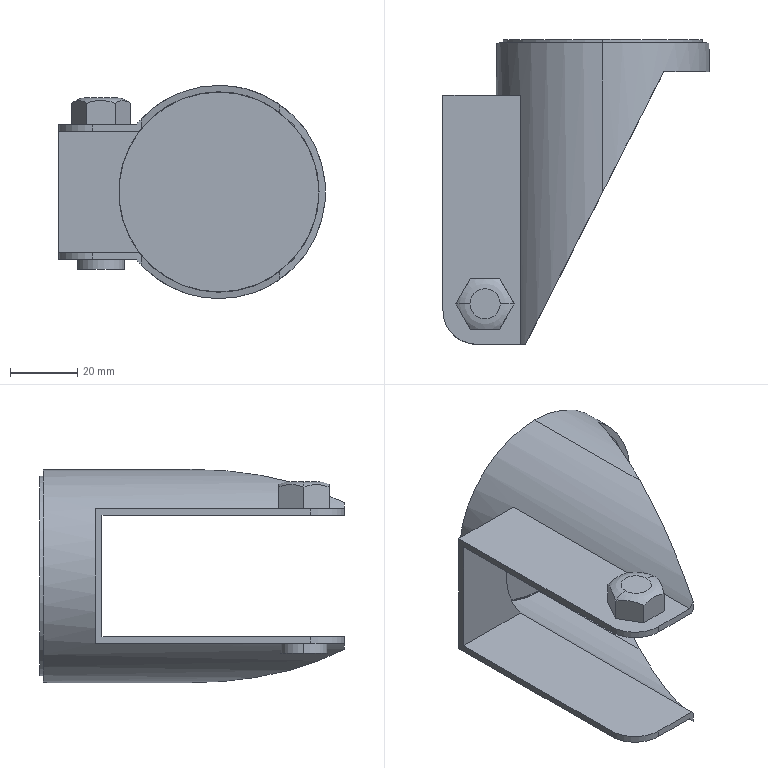Part | SolidWorks | features RefAxis 15, ICE 6, 3DProfileFeature 5, Revolution 2 | 1 solid | 38 faces | box 79.167 x 90.525 x 63.333 mm | volume 28539 mm3 | plane 24 | cylinder 12 | torus 2 | commonest cylinder face diameters 59.333 x4 14 x2 20 x2 59.533 x2 63.333 x2
STEP:
#1=CARTESIAN_POINT('',(-39.5,-94.,28.));
#2=VERTEX_POINT('',#1);
#3=CARTESIAN_POINT('',(-30.5,-94.,28.));
#4=VERTEX_POINT('',#3);
#5=CARTESIAN_POINT('',(-35.,-94.,28.));
#6=DIRECTION('',(0.,0.,-1.));
#7=DIRECTION('',(-1.,0.,0.));
#8=AXIS2_PLACEMENT_3D('',#5,#6,#7);
#9=CIRCLE('',#8,4.5);
#10=EDGE_CURVE('',#2,#4,#9,.T.);
#11=ORIENTED_EDGE('',*,*,#10,.T.);
#12=CARTESIAN_POINT('',(-26.34,-94.,26.33));
#13=VERTEX_POINT('',#12);
#14=CARTESIAN_POINT('',(-30.693,-94.,21.503));
#15=DIRECTION('',(0.,1.,0.));
#16=DIRECTION('',(-1.,0.,0.));
#17=AXIS2_PLACEMENT_3D('',#14,#15,#16);
#18=CIRCLE('',#17,6.5);
#19=EDGE_CURVE('',#4,#13,#18,.T.);
#20=ORIENTED_EDGE('',*,*,#19,.T.);
#21=CARTESIAN_POINT('',(-30.67,-86.5,26.33));
#22=VERTEX_POINT('',#21);
#23=CARTESIAN_POINT('',(-30.67,-86.5,26.33));
#24=CARTESIAN_POINT('',(-30.329,-87.091,26.637));
#25=CARTESIAN_POINT('',(-29.974,-87.705,26.84));
#26=CARTESIAN_POINT('',(-29.429,-88.65,27.038));
#27=CARTESIAN_POINT('',(-29.244,-88.97,27.086));
#28=CARTESIAN_POINT('',(-28.874,-89.611,27.149));
#29=CARTESIAN_POINT('',(-28.689,-89.931,27.164));
#30=CARTESIAN_POINT('',(-28.137,-90.888,27.164));
#31=CARTESIAN_POINT('',(-27.77,-91.522,27.106));
#32=CARTESIAN_POINT('',(-27.225,-92.467,26.909));
#33=CARTESIAN_POINT('',(-27.043,-92.783,26.825));
#34=CARTESIAN_POINT('',(-26.685,-93.402,26.611));
#35=CARTESIAN_POINT('',(-26.51,-93.705,26.483));
#36=CARTESIAN_POINT('',(-26.34,-94.,26.33));
#37=B_SPLINE_CURVE_WITH_KNOTS('',3,(#23,#24,#25,#26,#27,#28,#29,#30,#31,#32,#33,#34,#35,#36),.UNSPECIFIED.,.F.,.F.,(4,2,2,2,2,2,4),(0.00000025,0.002212,0.003318,0.004423,0.006635,0.007741,0.008847),.UNSPECIFIED.);
#38=EDGE_CURVE('',#22,#13,#37,.T.);
#39=ORIENTED_EDGE('',*,*,#38,.F.);
#40=CARTESIAN_POINT('',(-39.33,-86.5,26.33));
#41=VERTEX_POINT('',#40);
#42=CARTESIAN_POINT('',(-39.33,-86.5,26.33));
#43=CARTESIAN_POINT('',(-38.993,-86.5,26.482));
#44=CARTESIAN_POINT('',(-38.645,-86.5,26.61));
#45=CARTESIAN_POINT('',(-37.93,-86.5,26.823));
#46=CARTESIAN_POINT('',(-37.565,-86.5,26.908));
#47=CARTESIAN_POINT('',(-36.833,-86.5,27.04));
#48=CARTESIAN_POINT('',(-36.466,-86.5,27.088));
#49=CARTESIAN_POINT('',(-35.726,-86.5,27.15));
#50=CARTESIAN_POINT('',(-35.351,-86.5,27.165));
#51=CARTESIAN_POINT('',(-34.237,-86.5,27.163));
#52=CARTESIAN_POINT('',(-33.505,-86.5,27.103));
#53=CARTESIAN_POINT('',(-32.424,-86.5,26.906));
#54=CARTESIAN_POINT('',(-32.067,-86.5,26.822));
#55=CARTESIAN_POINT('',(-31.361,-86.5,26.611));
#56=CARTESIAN_POINT('',(-31.009,-86.5,26.483));
#57=CARTESIAN_POINT('',(-30.67,-86.5,26.33));
#58=B_SPLINE_CURVE_WITH_KNOTS('',3,(#42,#43,#44,#45,#46,#47,#48,#49,#50,#51,#52,#53,#54,#55,#56,#57),.UNSPECIFIED.,.F.,.F.,(4,2,2,2,2,2,2,4),(0.0379,0.039,0.0401,0.0412,0.04229,0.04449,0.04559,0.04669),.UNSPECIFIED.);
#59=EDGE_CURVE('',#41,#22,#58,.T.);
#60=ORIENTED_EDGE('',*,*,#59,.F.);
#61=CARTESIAN_POINT('',(-43.66,-94.,26.33));
#62=VERTEX_POINT('',#61);
#63=CARTESIAN_POINT('',(-43.66,-94.,26.33));
#64=CARTESIAN_POINT('',(-43.319,-93.409,26.637));
#65=CARTESIAN_POINT('',(-42.964,-92.795,26.84));
#66=CARTESIAN_POINT('',(-42.419,-91.85,27.038));
#67=CARTESIAN_POINT('',(-42.234,-91.53,27.086));
#68=CARTESIAN_POINT('',(-41.864,-90.889,27.149));
#69=CARTESIAN_POINT('',(-41.679,-90.569,27.164));
#70=CARTESIAN_POINT('',(-41.127,-89.612,27.164));
#71=CARTESIAN_POINT('',(-40.761,-88.978,27.106));
#72=CARTESIAN_POINT('',(-40.215,-88.033,26.909));
#73=CARTESIAN_POINT('',(-40.033,-87.717,26.825));
#74=CARTESIAN_POINT('',(-39.676,-87.098,26.611));
#75=CARTESIAN_POINT('',(-39.501,-86.795,26.483));
#76=CARTESIAN_POINT('',(-39.33,-86.5,26.33));
#77=B_SPLINE_CURVE_WITH_KNOTS('',3,(#63,#64,#65,#66,#67,#68,#69,#70,#71,#72,#73,#74,#75,#76),.UNSPECIFIED.,.F.,.F.,(4,2,2,2,2,2,4),(0.00000025,0.002212,0.003318,0.004423,0.006635,0.007741,0.008847),.UNSPECIFIED.);
#78=EDGE_CURVE('',#62,#41,#77,.T.);
#79=ORIENTED_EDGE('',*,*,#78,.F.);
#80=CARTESIAN_POINT('',(-39.307,-94.,21.503));
#81=DIRECTION('',(0.,-1.,0.));
#82=DIRECTION('',(0.,0.,-1.));
#83=AXIS2_PLACEMENT_3D('',#80,#81,#82);
#84=CIRCLE('',#83,6.5);
#85=EDGE_CURVE('',#2,#62,#84,.T.);
#86=ORIENTED_EDGE('',*,*,#85,.F.);
#87=EDGE_LOOP('',(#11,#20,#39,#60,#79,#86));
#88=FACE_OUTER_BOUND('',#87,.T.);
#89=CARTESIAN_POINT('',(-35.,-94.,21.503));
#90=DIRECTION('',(0.,0.,-1.));
#91=DIRECTION('',(-1.,0.,0.));
#92=AXIS2_PLACEMENT_3D('',#89,#90,#91);
#93=TOROIDAL_SURFACE('',#92,4.307,6.5);
#94=ADVANCED_FACE('',(#88),#93,.T.);
#95=CARTESIAN_POINT('',(-28.,-94.,-23.));
#96=VERTEX_POINT('',#95);
#97=CARTESIAN_POINT('',(-42.,-94.,-23.));
#98=VERTEX_POINT('',#97);
#99=CARTESIAN_POINT('',(-35.,-94.,-23.));
#100=DIRECTION('',(0.,0.,1.));
#101=DIRECTION('',(1.,0.,0.));
#102=AXIS2_PLACEMENT_3D('',#99,#100,#101);
#103=CIRCLE('',#102,7.);
#104=EDGE_CURVE('',#96,#98,#103,.T.);
#105=ORIENTED_EDGE('',*,*,#104,.T.);
#106=CARTESIAN_POINT('',(-42.,-94.,-20.));
#107=VERTEX_POINT('',#106);
#108=CARTESIAN_POINT('',(-42.,-94.,-23.));
#109=DIRECTION('',(0.,0.,1.));
#110=VECTOR('',#109,1000.);
#111=LINE('',#108,#110);
#112=EDGE_CURVE('',#98,#107,#111,.T.);
#113=ORIENTED_EDGE('',*,*,#112,.T.);
#114=CARTESIAN_POINT('',(-28.,-94.,-20.));
#115=VERTEX_POINT('',#114);
#116=CARTESIAN_POINT('',(-35.,-94.,-20.));
#117=DIRECTION('',(0.,0.,-1.));
#118=DIRECTION('',(-1.,0.,0.));
#119=AXIS2_PLACEMENT_3D('',#116,#117,#118);
#120=CIRCLE('',#119,7.);
#121=EDGE_CURVE('',#107,#115,#120,.T.);
#122=ORIENTED_EDGE('',*,*,#121,.T.);
#123=CARTESIAN_POINT('',(-28.,-94.,-23.));
#124=DIRECTION('',(0.,0.,1.));
#125=VECTOR('',#124,1000.);
#126=LINE('',#123,#125);
#127=EDGE_CURVE('',#96,#115,#126,.T.);
#128=ORIENTED_EDGE('',*,*,#127,.F.);
#129=EDGE_LOOP('',(#105,#113,#122,#128));
#130=FACE_OUTER_BOUND('',#129,.T.);
#131=CARTESIAN_POINT('',(-35.,-94.,-23.));
#132=DIRECTION('',(0.,0.,1.));
#133=DIRECTION('',(1.,0.,0.));
#134=AXIS2_PLACEMENT_3D('',#131,#132,#133);
#135=CYLINDRICAL_SURFACE('',#134,7.);
#136=ADVANCED_FACE('',(#130),#135,.T.);
#137=CARTESIAN_POINT('',(0.,-18.475,-29.667));
#138=VERTEX_POINT('',#137);
#139=CARTESIAN_POINT('',(0.,-18.475,29.667));
#140=VERTEX_POINT('',#139);
#141=CARTESIAN_POINT('',(0.,-18.475,0.));
#142=DIRECTION('',(0.,1.,0.));
#143=DIRECTION('',(0.,0.,1.));
#144=AXIS2_PLACEMENT_3D('',#141,#142,#143);
#145=CIRCLE('',#144,29.667);
#146=EDGE_CURVE('',#138,#140,#145,.T.);
#147=ORIENTED_EDGE('',*,*,#146,.F.);
#148=CARTESIAN_POINT('',(0.,-17.975,-29.667));
#149=VERTEX_POINT('',#148);
#150=CARTESIAN_POINT('',(0.,-15.475,-29.667));
#151=DIRECTION('',(0.,1.,0.));
#152=VECTOR('',#151,1000.);
#153=LINE('',#150,#152);
#154=EDGE_CURVE('',#138,#149,#153,.T.);
#155=ORIENTED_EDGE('',*,*,#154,.T.);
#156=CARTESIAN_POINT('',(0.,-17.975,29.667));
#157=VERTEX_POINT('',#156);
#158=CARTESIAN_POINT('',(0.,-17.975,0.));
#159=DIRECTION('',(0.,1.,0.));
#160=DIRECTION('',(0.,0.,1.));
#161=AXIS2_PLACEMENT_3D('',#158,#159,#160);
#162=CIRCLE('',#161,29.667);
#163=EDGE_CURVE('',#149,#157,#162,.T.);
#164=ORIENTED_EDGE('',*,*,#163,.T.);
#165=CARTESIAN_POINT('',(0.,-15.475,29.667));
#166=DIRECTION('',(0.,1.,0.));
#167=VECTOR('',#166,1000.);
#168=LINE('',#165,#167);
#169=EDGE_CURVE('',#140,#157,#168,.T.);
#170=ORIENTED_EDGE('',*,*,#169,.F.);
#171=EDGE_LOOP('',(#147,#155,#164,#170));
#172=FACE_OUTER_BOUND('',#171,.T.);
#173=CARTESIAN_POINT('',(0.,-15.475,0.));
#174=DIRECTION('',(0.,1.,0.));
#175=DIRECTION('',(0.,0.,1.));
#176=AXIS2_PLACEMENT_3D('',#173,#174,#175);
#177=CYLINDRICAL_SURFACE('',#176,29.667);
#178=ADVANCED_FACE('',(#172),#177,.F.);
#179=CARTESIAN_POINT('',(-23.03,-106.,-18.859));
#180=VERTEX_POINT('',#179);
#181=CARTESIAN_POINT('',(0.,-60.626,-29.767));
#182=VERTEX_POINT('',#181);
#183=CARTESIAN_POINT('',(-23.03,-106.,-18.859));
#184=CARTESIAN_POINT('',(-17.28,-94.67,-25.881));
#185=CARTESIAN_POINT('',(-9.077,-78.509,-29.767));
#186=CARTESIAN_POINT('',(0.,-60.626,-29.767));
#187=(BOUNDED_CURVE()B_SPLINE_CURVE(3,(#183,#184,#185,#186),.UNSPECIFIED.,.F.,.F.)B_SPLINE_CURVE_WITH_KNOTS((4,4),(3.828,4.712),.UNSPECIFIED.)CURVE()GEOMETRIC_REPRESENTATION_ITEM()RATIONAL_B_SPLINE_CURVE((1.,0.9358,0.9358,1.))REPRESENTATION_ITEM(''));
#188=EDGE_CURVE('',#180,#182,#187,.T.);
#189=ORIENTED_EDGE('',*,*,#188,.T.);
#190=CARTESIAN_POINT('',(0.,-18.475,-29.767));
#191=VERTEX_POINT('',#190);
#192=CARTESIAN_POINT('',(0.,-162.475,-29.767));
#193=DIRECTION('',(0.,1.,0.));
#194=VECTOR('',#193,1000.);
#195=LINE('',#192,#194);
#196=EDGE_CURVE('',#182,#191,#195,.T.);
#197=ORIENTED_EDGE('',*,*,#196,.T.);
#198=CARTESIAN_POINT('',(0.,-18.475,29.767));
#199=VERTEX_POINT('',#198);
#200=CARTESIAN_POINT('',(0.,-18.475,0.));
#201=DIRECTION('',(0.,1.,0.));
#202=DIRECTION('',(0.,0.,1.));
#203=AXIS2_PLACEMENT_3D('',#200,#201,#202);
#204=CIRCLE('',#203,29.767);
#205=EDGE_CURVE('',#191,#199,#204,.T.);
#206=ORIENTED_EDGE('',*,*,#205,.T.);
#207=CARTESIAN_POINT('',(0.,-60.626,29.767));
#208=VERTEX_POINT('',#207);
#209=CARTESIAN_POINT('',(0.,-162.475,29.767));
#210=DIRECTION('',(0.,1.,0.));
#211=VECTOR('',#210,1000.);
#212=LINE('',#209,#211);
#213=EDGE_CURVE('',#208,#199,#212,.T.);
#214=ORIENTED_EDGE('',*,*,#213,.F.);
#215=CARTESIAN_POINT('',(-23.03,-106.,18.859));
#216=VERTEX_POINT('',#215);
#217=CARTESIAN_POINT('',(0.,-60.626,29.767));
#218=CARTESIAN_POINT('',(-9.077,-78.509,29.767));
#219=CARTESIAN_POINT('',(-17.28,-94.67,25.881));
#220=CARTESIAN_POINT('',(-23.03,-106.,18.859));
#221=(BOUNDED_CURVE()B_SPLINE_CURVE(3,(#217,#218,#219,#220),.UNSPECIFIED.,.F.,.F.)B_SPLINE_CURVE_WITH_KNOTS((4,4),(1.571,2.455),.UNSPECIFIED.)CURVE()GEOMETRIC_REPRESENTATION_ITEM()RATIONAL_B_SPLINE_CURVE((1.,0.9358,0.9358,1.))REPRESENTATION_ITEM(''));
#222=EDGE_CURVE('',#208,#216,#221,.T.);
#223=ORIENTED_EDGE('',*,*,#222,.T.);
#224=CARTESIAN_POINT('',(-23.708,-106.,18.));
#225=VERTEX_POINT('',#224);
#226=CARTESIAN_POINT('',(0.,-106.,0.));
#227=DIRECTION('',(0.,-1.,0.));
#228=DIRECTION('',(0.,0.,1.));
#229=AXIS2_PLACEMENT_3D('',#226,#227,#228);
#230=CIRCLE('',#229,29.767);
#231=EDGE_CURVE('',#216,#225,#230,.T.);
#232=ORIENTED_EDGE('',*,*,#231,.T.);
#233=CARTESIAN_POINT('',(-23.708,-34.,18.));
#234=VERTEX_POINT('',#233);
#235=CARTESIAN_POINT('',(-23.708,-162.475,18.));
#236=DIRECTION('',(0.,-1.,0.));
#237=VECTOR('',#236,1000.);
#238=LINE('',#235,#237);
#239=EDGE_CURVE('',#234,#225,#238,.T.);
#240=ORIENTED_EDGE('',*,*,#239,.F.);
#241=CARTESIAN_POINT('',(-23.708,-34.,-18.));
#242=VERTEX_POINT('',#241);
#243=CARTESIAN_POINT('',(0.,-34.,0.));
#244=DIRECTION('',(0.,1.,0.));
#245=DIRECTION('',(0.,0.,1.));
#246=AXIS2_PLACEMENT_3D('',#243,#244,#245);
#247=CIRCLE('',#246,29.767);
#248=EDGE_CURVE('',#242,#234,#247,.T.);
#249=ORIENTED_EDGE('',*,*,#248,.F.);
#250=CARTESIAN_POINT('',(-23.708,-106.,-18.));
#251=VERTEX_POINT('',#250);
#252=CARTESIAN_POINT('',(-23.708,-162.475,-18.));
#253=DIRECTION('',(0.,1.,0.));
#254=VECTOR('',#253,1000.);
#255=LINE('',#252,#254);
#256=EDGE_CURVE('',#251,#242,#255,.T.);
#257=ORIENTED_EDGE('',*,*,#256,.F.);
#258=CARTESIAN_POINT('',(0.,-106.,0.));
#259=DIRECTION('',(0.,-1.,0.));
#260=DIRECTION('',(0.,0.,1.));
#261=AXIS2_PLACEMENT_3D('',#258,#259,#260);
#262=CIRCLE('',#261,29.767);
#263=EDGE_CURVE('',#251,#180,#262,.T.);
#264=ORIENTED_EDGE('',*,*,#263,.T.);
#265=EDGE_LOOP('',(#189,#197,#206,#214,#223,#232,#240,#249,#257,#264));
#266=FACE_OUTER_BOUND('',#265,.T.);
#267=CARTESIAN_POINT('',(0.,-162.475,0.));
#268=DIRECTION('',(0.,1.,0.));
#269=DIRECTION('',(0.,0.,1.));
#270=AXIS2_PLACEMENT_3D('',#267,#268,#269);
#271=CYLINDRICAL_SURFACE('',#270,29.767);
#272=ADVANCED_FACE('',(#266),#271,.F.);
#273=CARTESIAN_POINT('',(0.,-16.475,29.667));
#274=VERTEX_POINT('',#273);
#275=CARTESIAN_POINT('',(0.,-16.475,-29.667));
#276=VERTEX_POINT('',#275);
#277=CARTESIAN_POINT('',(0.,-16.475,0.));
#278=DIRECTION('',(0.,1.,0.));
#279=DIRECTION('',(0.,0.,1.));
#280=AXIS2_PLACEMENT_3D('',#277,#278,#279);
#281=CIRCLE('',#280,29.667);
#282=EDGE_CURVE('',#274,#276,#281,.T.);
#283=ORIENTED_EDGE('',*,*,#282,.T.);
#284=CARTESIAN_POINT('',(0.,-15.475,-29.667));
#285=VERTEX_POINT('',#284);
#286=CARTESIAN_POINT('',(0.,-15.475,-29.667));
#287=DIRECTION('',(0.,1.,0.));
#288=VECTOR('',#287,1000.);
#289=LINE('',#286,#288);
#290=EDGE_CURVE('',#276,#285,#289,.T.);
#291=ORIENTED_EDGE('',*,*,#290,.T.);
#292=CARTESIAN_POINT('',(0.,-15.475,29.667));
#293=VERTEX_POINT('',#292);
#294=CARTESIAN_POINT('',(0.,-15.475,0.));
#295=DIRECTION('',(0.,1.,0.));
#296=DIRECTION('',(0.,0.,1.));
#297=AXIS2_PLACEMENT_3D('',#294,#295,#296);
#298=CIRCLE('',#297,29.667);
#299=EDGE_CURVE('',#293,#285,#298,.T.);
#300=ORIENTED_EDGE('',*,*,#299,.F.);
#301=CARTESIAN_POINT('',(0.,-15.475,29.667));
#302=DIRECTION('',(0.,1.,0.));
#303=VECTOR('',#302,1000.);
#304=LINE('',#301,#303);
#305=EDGE_CURVE('',#274,#293,#304,.T.);
#306=ORIENTED_EDGE('',*,*,#305,.F.);
#307=EDGE_LOOP('',(#283,#291,#300,#306));
#308=FACE_OUTER_BOUND('',#307,.T.);
#309=CARTESIAN_POINT('',(0.,-15.475,0.));
#310=DIRECTION('',(0.,1.,0.));
#311=DIRECTION('',(0.,0.,1.));
#312=AXIS2_PLACEMENT_3D('',#309,#310,#311);
#313=CYLINDRICAL_SURFACE('',#312,29.667);
#314=ADVANCED_FACE('',(#308),#313,.T.);
#315=CARTESIAN_POINT('',(0.,-60.626,-31.667));
#316=VERTEX_POINT('',#315);
#317=CARTESIAN_POINT('',(18.095,-24.975,-25.987));
#318=VERTEX_POINT('',#317);
#319=CARTESIAN_POINT('',(0.,-60.626,-31.667));
#320=CARTESIAN_POINT('',(6.521,-47.778,-31.667));
#321=CARTESIAN_POINT('',(12.743,-35.519,-29.714));
#322=CARTESIAN_POINT('',(18.095,-24.975,-25.987));
#323=(BOUNDED_CURVE()B_SPLINE_CURVE(3,(#319,#320,#321,#322),.UNSPECIFIED.,.F.,.T.)B_SPLINE_CURVE_WITH_KNOTS((4,4),(4.712,5.321),.UNSPECIFIED.)CURVE()GEOMETRIC_REPRESENTATION_ITEM()RATIONAL_B_SPLINE_CURVE((1.,0.9694,0.9694,1.))REPRESENTATION_ITEM(''));
#324=EDGE_CURVE('',#316,#318,#323,.T.);
#325=ORIENTED_EDGE('',*,*,#324,.F.);
#326=CARTESIAN_POINT('',(0.,-16.475,-31.667));
#327=VERTEX_POINT('',#326);
#328=CARTESIAN_POINT('',(0.,-15.475,-31.667));
#329=DIRECTION('',(0.,1.,0.));
#330=VECTOR('',#329,1000.);
#331=LINE('',#328,#330);
#332=EDGE_CURVE('',#316,#327,#331,.T.);
#333=ORIENTED_EDGE('',*,*,#332,.T.);
#334=CARTESIAN_POINT('',(0.,-16.475,31.667));
#335=VERTEX_POINT('',#334);
#336=CARTESIAN_POINT('',(0.,-16.475,0.));
#337=DIRECTION('',(0.,1.,0.));
#338=DIRECTION('',(0.,0.,1.));
#339=AXIS2_PLACEMENT_3D('',#336,#337,#338);
#340=CIRCLE('',#339,31.667);
#341=EDGE_CURVE('',#335,#327,#340,.T.);
#342=ORIENTED_EDGE('',*,*,#341,.F.);
#343=CARTESIAN_POINT('',(0.,-60.626,31.667));
#344=VERTEX_POINT('',#343);
#345=CARTESIAN_POINT('',(0.,-15.475,31.667));
#346=DIRECTION('',(0.,1.,0.));
#347=VECTOR('',#346,1000.);
#348=LINE('',#345,#347);
#349=EDGE_CURVE('',#344,#335,#348,.T.);
#350=ORIENTED_EDGE('',*,*,#349,.F.);
#351=CARTESIAN_POINT('',(18.095,-24.975,25.987));
#352=VERTEX_POINT('',#351);
#353=CARTESIAN_POINT('',(18.095,-24.975,25.987));
#354=CARTESIAN_POINT('',(12.743,-35.519,29.714));
#355=CARTESIAN_POINT('',(6.521,-47.778,31.667));
#356=CARTESIAN_POINT('',(0.,-60.626,31.667));
#357=(BOUNDED_CURVE()B_SPLINE_CURVE(3,(#353,#354,#355,#356),.UNSPECIFIED.,.F.,.F.)B_SPLINE_CURVE_WITH_KNOTS((4,4),(0.9626,1.571),.UNSPECIFIED.)CURVE()GEOMETRIC_REPRESENTATION_ITEM()RATIONAL_B_SPLINE_CURVE((1.,0.9694,0.9694,1.))REPRESENTATION_ITEM(''));
#358=EDGE_CURVE('',#352,#344,#357,.T.);
#359=ORIENTED_EDGE('',*,*,#358,.F.);
#360=CARTESIAN_POINT('',(0.,-24.975,0.));
#361=DIRECTION('',(0.,-1.,0.));
#362=DIRECTION('',(-1.,0.,0.));
#363=AXIS2_PLACEMENT_3D('',#360,#361,#362);
#364=CIRCLE('',#363,31.667);
#365=EDGE_CURVE('',#318,#352,#364,.T.);
#366=ORIENTED_EDGE('',*,*,#365,.F.);
#367=EDGE_LOOP('',(#325,#333,#342,#350,#359,#366));
#368=FACE_OUTER_BOUND('',#367,.T.);
#369=CARTESIAN_POINT('',(0.,-15.475,0.));
#370=DIRECTION('',(0.,1.,0.));
#371=DIRECTION('',(0.,0.,1.));
#372=AXIS2_PLACEMENT_3D('',#369,#370,#371);
#373=CYLINDRICAL_SURFACE('',#372,31.667);
#374=ADVANCED_FACE('',(#368),#373,.T.);
#375=CARTESIAN_POINT('',(-47.5,-32.,-20.));
#376=VERTEX_POINT('',#375);
#377=CARTESIAN_POINT('',(-47.5,-32.,20.));
#378=VERTEX_POINT('',#377);
#379=CARTESIAN_POINT('',(-47.5,-32.,-20.));
#380=DIRECTION('',(0.,0.,1.));
#381=VECTOR('',#380,1000.);
#382=LINE('',#379,#381);
#383=EDGE_CURVE('',#376,#378,#382,.T.);
#384=ORIENTED_EDGE('',*,*,#383,.F.);
#385=CARTESIAN_POINT('',(-47.5,-96.,-20.));
#386=VERTEX_POINT('',#385);
#387=CARTESIAN_POINT('',(-47.5,-106.,-20.));
#388=DIRECTION('',(0.,1.,0.));
#389=VECTOR('',#388,1000.);
#390=LINE('',#387,#389);
#391=EDGE_CURVE('',#386,#376,#390,.T.);
#392=ORIENTED_EDGE('',*,*,#391,.F.);
#393=CARTESIAN_POINT('',(-47.5,-96.,-18.));
#394=VERTEX_POINT('',#393);
#395=CARTESIAN_POINT('',(-47.5,-96.,-95.));
#396=DIRECTION('',(0.,0.,1.));
#397=VECTOR('',#396,1000.);
#398=LINE('',#395,#397);
#399=EDGE_CURVE('',#386,#394,#398,.T.);
#400=ORIENTED_EDGE('',*,*,#399,.T.);
#401=CARTESIAN_POINT('',(-47.5,-34.,-18.));
#402=VERTEX_POINT('',#401);
#403=CARTESIAN_POINT('',(-47.5,-34.,-18.));
#404=DIRECTION('',(0.,-1.,0.));
#405=VECTOR('',#404,1000.);
#406=LINE('',#403,#405);
#407=EDGE_CURVE('',#402,#394,#406,.T.);
#408=ORIENTED_EDGE('',*,*,#407,.F.);
#409=CARTESIAN_POINT('',(-47.5,-34.,18.));
#410=VERTEX_POINT('',#409);
#411=CARTESIAN_POINT('',(-47.5,-34.,18.));
#412=DIRECTION('',(0.,0.,-1.));
#413=VECTOR('',#412,1000.);
#414=LINE('',#411,#413);
#415=EDGE_CURVE('',#410,#402,#414,.T.);
#416=ORIENTED_EDGE('',*,*,#415,.F.);
#417=CARTESIAN_POINT('',(-47.5,-96.,18.));
#418=VERTEX_POINT('',#417);
#419=CARTESIAN_POINT('',(-47.5,-106.,18.));
#420=DIRECTION('',(0.,1.,0.));
#421=VECTOR('',#420,1000.);
#422=LINE('',#419,#421);
#423=EDGE_CURVE('',#418,#410,#422,.T.);
#424=ORIENTED_EDGE('',*,*,#423,.F.);
#425=CARTESIAN_POINT('',(-47.5,-96.,20.));
#426=VERTEX_POINT('',#425);
#427=CARTESIAN_POINT('',(-47.5,-96.,-95.));
#428=DIRECTION('',(0.,0.,1.));
#429=VECTOR('',#428,1000.);
#430=LINE('',#427,#429);
#431=EDGE_CURVE('',#418,#426,#430,.T.);
#432=ORIENTED_EDGE('',*,*,#431,.T.);
#433=CARTESIAN_POINT('',(-47.5,-32.,20.));
#434=DIRECTION('',(0.,-1.,0.));
#435=VECTOR('',#434,1000.);
#436=LINE('',#433,#435);
#437=EDGE_CURVE('',#378,#426,#436,.T.);
#438=ORIENTED_EDGE('',*,*,#437,.F.);
#439=EDGE_LOOP('',(#384,#392,#400,#408,#416,#424,#432,#438));
#440=FACE_OUTER_BOUND('',#439,.T.);
#441=CARTESIAN_POINT('',(-47.5,0.,0.));
#442=DIRECTION('',(1.,0.,0.));
#443=DIRECTION('',(0.,0.,-1.));
#444=AXIS2_PLACEMENT_3D('',#441,#442,#443);
#445=PLANE('',#444);
#446=ADVANCED_FACE('',(#440),#445,.F.);
#447=CARTESIAN_POINT('',(-37.5,-106.,20.));
#448=VERTEX_POINT('',#447);
#449=CARTESIAN_POINT('',(-24.552,-106.,20.));
#450=VERTEX_POINT('',#449);
#451=CARTESIAN_POINT('',(-47.5,-106.,20.));
#452=DIRECTION('',(1.,0.,0.));
#453=VECTOR('',#452,1000.);
#454=LINE('',#451,#453);
#455=EDGE_CURVE('',#448,#450,#454,.T.);
#456=ORIENTED_EDGE('',*,*,#455,.F.);
#457=CARTESIAN_POINT('',(-37.5,-106.,18.));
#458=VERTEX_POINT('',#457);
#459=CARTESIAN_POINT('',(-37.5,-106.,-95.));
#460=DIRECTION('',(0.,0.,1.));
#461=VECTOR('',#460,1000.);
#462=LINE('',#459,#461);
#463=EDGE_CURVE('',#458,#448,#462,.T.);
#464=ORIENTED_EDGE('',*,*,#463,.F.);
#465=CARTESIAN_POINT('',(-47.5,-106.,18.));
#466=DIRECTION('',(1.,0.,0.));
#467=VECTOR('',#466,1000.);
#468=LINE('',#465,#467);
#469=EDGE_CURVE('',#458,#225,#468,.T.);
#470=ORIENTED_EDGE('',*,*,#469,.T.);
#471=ORIENTED_EDGE('',*,*,#231,.F.);
#472=CARTESIAN_POINT('',(-23.03,-106.,21.734));
#473=VERTEX_POINT('',#472);
#474=CARTESIAN_POINT('',(-23.03,-106.,-95.));
#475=DIRECTION('',(0.,0.,1.));
#476=VECTOR('',#475,1000.);
#477=LINE('',#474,#476);
#478=EDGE_CURVE('',#216,#473,#477,.T.);
#479=ORIENTED_EDGE('',*,*,#478,.T.);
#480=CARTESIAN_POINT('',(0.,-106.,0.));
#481=DIRECTION('',(0.,-1.,0.));
#482=DIRECTION('',(0.,0.,1.));
#483=AXIS2_PLACEMENT_3D('',#480,#481,#482);
#484=CIRCLE('',#483,31.667);
#485=EDGE_CURVE('',#473,#450,#484,.T.);
#486=ORIENTED_EDGE('',*,*,#485,.T.);
#487=EDGE_LOOP('',(#456,#464,#470,#471,#479,#486));
#488=FACE_OUTER_BOUND('',#487,.T.);
#489=CARTESIAN_POINT('',(-47.5,-106.,20.));
#490=DIRECTION('',(0.,-1.,0.));
#491=DIRECTION('',(0.,0.,-1.));
#492=AXIS2_PLACEMENT_3D('',#489,#490,#491);
#493=PLANE('',#492);
#494=ADVANCED_FACE('',(#488),#493,.T.);
#495=CARTESIAN_POINT('',(-37.5,-106.,-18.));
#496=VERTEX_POINT('',#495);
#497=CARTESIAN_POINT('',(-47.5,-106.,-18.));
#498=DIRECTION('',(1.,0.,0.));
#499=VECTOR('',#498,1000.);
#500=LINE('',#497,#499);
#501=EDGE_CURVE('',#496,#251,#500,.T.);
#502=ORIENTED_EDGE('',*,*,#501,.F.);
#503=CARTESIAN_POINT('',(-37.5,-106.,-20.));
#504=VERTEX_POINT('',#503);
#505=CARTESIAN_POINT('',(-37.5,-106.,-95.));
#506=DIRECTION('',(0.,0.,1.));
#507=VECTOR('',#506,1000.);
#508=LINE('',#505,#507);
#509=EDGE_CURVE('',#504,#496,#508,.T.);
#510=ORIENTED_EDGE('',*,*,#509,.F.);
#511=CARTESIAN_POINT('',(-24.552,-106.,-20.));
#512=VERTEX_POINT('',#511);
#513=CARTESIAN_POINT('',(-47.5,-106.,-20.));
#514=DIRECTION('',(1.,0.,0.));
#515=VECTOR('',#514,1000.);
#516=LINE('',#513,#515);
#517=EDGE_CURVE('',#504,#512,#516,.T.);
#518=ORIENTED_EDGE('',*,*,#517,.T.);
#519=CARTESIAN_POINT('',(-23.03,-106.,-21.734));
#520=VERTEX_POINT('',#519);
#521=CARTESIAN_POINT('',(0.,-106.,0.));
#522=DIRECTION('',(0.,-1.,0.));
#523=DIRECTION('',(0.,0.,1.));
#524=AXIS2_PLACEMENT_3D('',#521,#522,#523);
#525=CIRCLE('',#524,31.667);
#526=EDGE_CURVE('',#512,#520,#525,.T.);
#527=ORIENTED_EDGE('',*,*,#526,.T.);
#528=CARTESIAN_POINT('',(-23.03,-106.,-95.));
#529=DIRECTION('',(0.,0.,1.));
#530=VECTOR('',#529,1000.);
#531=LINE('',#528,#530);
#532=EDGE_CURVE('',#520,#180,#531,.T.);
#533=ORIENTED_EDGE('',*,*,#532,.T.);
#534=ORIENTED_EDGE('',*,*,#263,.F.);
#535=EDGE_LOOP('',(#502,#510,#518,#527,#533,#534));
#536=FACE_OUTER_BOUND('',#535,.T.);
#537=CARTESIAN_POINT('',(-47.5,-106.,-18.));
#538=DIRECTION('',(0.,-1.,0.));
#539=DIRECTION('',(0.,0.,-1.));
#540=AXIS2_PLACEMENT_3D('',#537,#538,#539);
#541=PLANE('',#540);
#542=ADVANCED_FACE('',(#536),#541,.T.);
#543=ORIENTED_EDGE('',*,*,#332,.F.);
#544=CARTESIAN_POINT('',(-23.03,-106.,-21.734));
#545=CARTESIAN_POINT('',(-16.961,-94.043,-28.165));
#546=CARTESIAN_POINT('',(-8.842,-78.047,-31.667));
#547=CARTESIAN_POINT('',(0.,-60.626,-31.667));
#548=(BOUNDED_CURVE()B_SPLINE_CURVE(3,(#544,#545,#546,#547),.UNSPECIFIED.,.F.,.T.)B_SPLINE_CURVE_WITH_KNOTS((4,4),(3.898,4.712),.UNSPECIFIED.)CURVE()GEOMETRIC_REPRESENTATION_ITEM()RATIONAL_B_SPLINE_CURVE((1.,0.9455,0.9455,1.))REPRESENTATION_ITEM(''));
#549=EDGE_CURVE('',#520,#316,#548,.T.);
#550=ORIENTED_EDGE('',*,*,#549,.F.);
#551=ORIENTED_EDGE('',*,*,#526,.F.);
#552=CARTESIAN_POINT('',(-24.552,-32.,-20.));
#553=VERTEX_POINT('',#552);
#554=CARTESIAN_POINT('',(-24.552,-15.475,-20.));
#555=DIRECTION('',(0.,-1.,0.));
#556=VECTOR('',#555,1000.);
#557=LINE('',#554,#556);
#558=EDGE_CURVE('',#553,#512,#557,.T.);
#559=ORIENTED_EDGE('',*,*,#558,.F.);
#560=CARTESIAN_POINT('',(-24.552,-32.,20.));
#561=VERTEX_POINT('',#560);
#562=CARTESIAN_POINT('',(0.,-32.,0.));
#563=DIRECTION('',(0.,-1.,0.));
#564=DIRECTION('',(0.,0.,1.));
#565=AXIS2_PLACEMENT_3D('',#562,#563,#564);
#566=CIRCLE('',#565,31.667);
#567=EDGE_CURVE('',#561,#553,#566,.T.);
#568=ORIENTED_EDGE('',*,*,#567,.F.);
#569=CARTESIAN_POINT('',(-24.552,-15.475,20.));
#570=DIRECTION('',(0.,1.,0.));
#571=VECTOR('',#570,1000.);
#572=LINE('',#569,#571);
#573=EDGE_CURVE('',#450,#561,#572,.T.);
#574=ORIENTED_EDGE('',*,*,#573,.F.);
#575=ORIENTED_EDGE('',*,*,#485,.F.);
#576=CARTESIAN_POINT('',(0.,-60.626,31.667));
#577=CARTESIAN_POINT('',(-8.842,-78.047,31.667));
#578=CARTESIAN_POINT('',(-16.961,-94.043,28.165));
#579=CARTESIAN_POINT('',(-23.03,-106.,21.734));
#580=(BOUNDED_CURVE()B_SPLINE_CURVE(3,(#576,#577,#578,#579),.UNSPECIFIED.,.F.,.F.)B_SPLINE_CURVE_WITH_KNOTS((4,4),(1.571,2.385),.UNSPECIFIED.)CURVE()GEOMETRIC_REPRESENTATION_ITEM()RATIONAL_B_SPLINE_CURVE((1.,0.9455,0.9455,1.))REPRESENTATION_ITEM(''));
#581=EDGE_CURVE('',#344,#473,#580,.T.);
#582=ORIENTED_EDGE('',*,*,#581,.F.);
#583=ORIENTED_EDGE('',*,*,#349,.T.);
#584=CARTESIAN_POINT('',(0.,-16.475,0.));
#585=DIRECTION('',(0.,1.,0.));
#586=DIRECTION('',(0.,0.,1.));
#587=AXIS2_PLACEMENT_3D('',#584,#585,#586);
#588=CIRCLE('',#587,31.667);
#589=EDGE_CURVE('',#327,#335,#588,.T.);
#590=ORIENTED_EDGE('',*,*,#589,.F.);
#591=EDGE_LOOP('',(#543,#550,#551,#559,#568,#574,#575,#582,#583,#590));
#592=FACE_OUTER_BOUND('',#591,.T.);
#593=CARTESIAN_POINT('',(0.,-15.475,0.));
#594=DIRECTION('',(0.,1.,0.));
#595=DIRECTION('',(0.,0.,1.));
#596=AXIS2_PLACEMENT_3D('',#593,#594,#595);
#597=CYLINDRICAL_SURFACE('',#596,31.667);
#598=ADVANCED_FACE('',(#592),#597,.T.);
#599=ORIENTED_EDGE('',*,*,#341,.T.);
#600=ORIENTED_EDGE('',*,*,#589,.T.);
#601=EDGE_LOOP('',(#599,#600));
#602=FACE_OUTER_BOUND('',#601,.T.);
#603=ORIENTED_EDGE('',*,*,#282,.F.);
#604=CARTESIAN_POINT('',(0.,-16.475,0.));
#605=DIRECTION('',(0.,1.,0.));
#606=DIRECTION('',(0.,0.,1.));
#607=AXIS2_PLACEMENT_3D('',#604,#605,#606);
#608=CIRCLE('',#607,29.667);
#609=EDGE_CURVE('',#276,#274,#608,.T.);
#610=ORIENTED_EDGE('',*,*,#609,.F.);
#611=EDGE_LOOP('',(#603,#610));
#612=FACE_BOUND('',#611,.T.);
#613=CARTESIAN_POINT('',(0.,-16.475,31.667));
#614=DIRECTION('',(0.,1.,0.));
#615=DIRECTION('',(0.,0.,1.));
#616=AXIS2_PLACEMENT_3D('',#613,#614,#615);
#617=PLANE('',#616);
#618=ADVANCED_FACE('',(#602,#612),#617,.T.);
#619=ORIENTED_EDGE('',*,*,#290,.F.);
#620=ORIENTED_EDGE('',*,*,#609,.T.);
#621=ORIENTED_EDGE('',*,*,#305,.T.);
#622=CARTESIAN_POINT('',(0.,-15.475,0.));
#623=DIRECTION('',(0.,1.,0.));
#624=DIRECTION('',(0.,0.,1.));
#625=AXIS2_PLACEMENT_3D('',#622,#623,#624);
#626=CIRCLE('',#625,29.667);
#627=EDGE_CURVE('',#285,#293,#626,.T.);
#628=ORIENTED_EDGE('',*,*,#627,.F.);
#629=EDGE_LOOP('',(#619,#620,#621,#628));
#630=FACE_OUTER_BOUND('',#629,.T.);
#631=CARTESIAN_POINT('',(0.,-15.475,0.));
#632=DIRECTION('',(0.,1.,0.));
#633=DIRECTION('',(0.,0.,1.));
#634=AXIS2_PLACEMENT_3D('',#631,#632,#633);
#635=CYLINDRICAL_SURFACE('',#634,29.667);
#636=ADVANCED_FACE('',(#630),#635,.T.);
#637=ORIENTED_EDGE('',*,*,#299,.T.);
#638=ORIENTED_EDGE('',*,*,#627,.T.);
#639=EDGE_LOOP('',(#637,#638));
#640=FACE_OUTER_BOUND('',#639,.T.);
#641=CARTESIAN_POINT('',(0.,-15.475,29.667));
#642=DIRECTION('',(0.,1.,0.));
#643=DIRECTION('',(0.,0.,1.));
#644=AXIS2_PLACEMENT_3D('',#641,#642,#643);
#645=PLANE('',#644);
#646=ADVANCED_FACE('',(#640),#645,.T.);
#647=CARTESIAN_POINT('',(-95.,-34.,-18.));
#648=DIRECTION('',(1.,0.,0.));
#649=VECTOR('',#648,1000.);
#650=LINE('',#647,#649);
#651=EDGE_CURVE('',#402,#242,#650,.T.);
#652=ORIENTED_EDGE('',*,*,#651,.T.);
#653=ORIENTED_EDGE('',*,*,#248,.T.);
#654=CARTESIAN_POINT('',(-95.,-34.,18.));
#655=DIRECTION('',(1.,0.,0.));
#656=VECTOR('',#655,1000.);
#657=LINE('',#654,#656);
#658=EDGE_CURVE('',#410,#234,#657,.T.);
#659=ORIENTED_EDGE('',*,*,#658,.F.);
#660=ORIENTED_EDGE('',*,*,#415,.T.);
#661=EDGE_LOOP('',(#652,#653,#659,#660));
#662=FACE_OUTER_BOUND('',#661,.T.);
#663=CARTESIAN_POINT('',(-95.,-34.,-18.));
#664=DIRECTION('',(0.,1.,0.));
#665=DIRECTION('',(0.,0.,1.));
#666=AXIS2_PLACEMENT_3D('',#663,#664,#665);
#667=PLANE('',#666);
#668=ADVANCED_FACE('',(#662),#667,.F.);
#669=ORIENTED_EDGE('',*,*,#407,.T.);
#670=CARTESIAN_POINT('',(-37.5,-96.,-18.));
#671=DIRECTION('',(0.,0.,1.));
#672=DIRECTION('',(-1.,0.,0.));
#673=AXIS2_PLACEMENT_3D('',#670,#671,#672);
#674=CIRCLE('',#673,10.);
#675=EDGE_CURVE('',#394,#496,#674,.T.);
#676=ORIENTED_EDGE('',*,*,#675,.T.);
#677=ORIENTED_EDGE('',*,*,#501,.T.);
#678=ORIENTED_EDGE('',*,*,#256,.T.);
#679=ORIENTED_EDGE('',*,*,#651,.F.);
#680=EDGE_LOOP('',(#669,#676,#677,#678,#679));
#681=FACE_OUTER_BOUND('',#680,.T.);
#682=CARTESIAN_POINT('',(-95.,-140.,-18.));
#683=DIRECTION('',(0.,0.,-1.));
#684=DIRECTION('',(-1.,0.,0.));
#685=AXIS2_PLACEMENT_3D('',#682,#683,#684);
#686=PLANE('',#685);
#687=ADVANCED_FACE('',(#681),#686,.F.);
#688=ORIENTED_EDGE('',*,*,#469,.F.);
#689=CARTESIAN_POINT('',(-37.5,-96.,18.));
#690=DIRECTION('',(0.,0.,-1.));
#691=DIRECTION('',(1.,0.,0.));
#692=AXIS2_PLACEMENT_3D('',#689,#690,#691);
#693=CIRCLE('',#692,10.);
#694=EDGE_CURVE('',#458,#418,#693,.T.);
#695=ORIENTED_EDGE('',*,*,#694,.T.);
#696=ORIENTED_EDGE('',*,*,#423,.T.);
#697=ORIENTED_EDGE('',*,*,#658,.T.);
#698=ORIENTED_EDGE('',*,*,#239,.T.);
#699=EDGE_LOOP('',(#688,#695,#696,#697,#698));
#700=FACE_OUTER_BOUND('',#699,.T.);
#701=CARTESIAN_POINT('',(-95.,-34.,18.));
#702=DIRECTION('',(0.,0.,1.));
#703=DIRECTION('',(1.,0.,0.));
#704=AXIS2_PLACEMENT_3D('',#701,#702,#703);
#705=PLANE('',#704);
#706=ADVANCED_FACE('',(#700),#705,.F.);
#707=CARTESIAN_POINT('',(-37.5,-96.,20.));
#708=DIRECTION('',(0.,0.,-1.));
#709=DIRECTION('',(1.,0.,0.));
#710=AXIS2_PLACEMENT_3D('',#707,#708,#709);
#711=CIRCLE('',#710,10.);
#712=EDGE_CURVE('',#448,#426,#711,.T.);
#713=ORIENTED_EDGE('',*,*,#712,.F.);
#714=ORIENTED_EDGE('',*,*,#455,.T.);
#715=ORIENTED_EDGE('',*,*,#573,.T.);
#716=CARTESIAN_POINT('',(-47.5,-32.,20.));
#717=DIRECTION('',(1.,0.,0.));
#718=VECTOR('',#717,1000.);
#719=LINE('',#716,#718);
#720=EDGE_CURVE('',#378,#561,#719,.T.);
#721=ORIENTED_EDGE('',*,*,#720,.F.);
#722=ORIENTED_EDGE('',*,*,#437,.T.);
#723=EDGE_LOOP('',(#713,#714,#715,#721,#722));
#724=FACE_OUTER_BOUND('',#723,.T.);
#725=CARTESIAN_POINT('',(-39.33,-86.5,20.));
#726=VERTEX_POINT('',#725);
#727=CARTESIAN_POINT('',(-43.66,-94.,20.));
#728=VERTEX_POINT('',#727);
#729=CARTESIAN_POINT('',(-39.33,-86.5,20.));
#730=DIRECTION('',(-0.5,-0.866,0.));
#731=VECTOR('',#730,1000.);
#732=LINE('',#729,#731);
#733=EDGE_CURVE('',#726,#728,#732,.T.);
#734=ORIENTED_EDGE('',*,*,#733,.F.);
#735=CARTESIAN_POINT('',(-30.67,-86.5,20.));
#736=VERTEX_POINT('',#735);
#737=CARTESIAN_POINT('',(-30.67,-86.5,20.));
#738=DIRECTION('',(-1.,0.,0.));
#739=VECTOR('',#738,1000.);
#740=LINE('',#737,#739);
#741=EDGE_CURVE('',#736,#726,#740,.T.);
#742=ORIENTED_EDGE('',*,*,#741,.F.);
#743=CARTESIAN_POINT('',(-26.34,-94.,20.));
#744=VERTEX_POINT('',#743);
#745=CARTESIAN_POINT('',(-26.34,-94.,20.));
#746=DIRECTION('',(-0.5,0.866,0.));
#747=VECTOR('',#746,1000.);
#748=LINE('',#745,#747);
#749=EDGE_CURVE('',#744,#736,#748,.T.);
#750=ORIENTED_EDGE('',*,*,#749,.F.);
#751=CARTESIAN_POINT('',(-30.67,-101.5,20.));
#752=VERTEX_POINT('',#751);
#753=CARTESIAN_POINT('',(-30.67,-101.5,20.));
#754=DIRECTION('',(0.5,0.866,0.));
#755=VECTOR('',#754,1000.);
#756=LINE('',#753,#755);
#757=EDGE_CURVE('',#752,#744,#756,.T.);
#758=ORIENTED_EDGE('',*,*,#757,.F.);
#759=CARTESIAN_POINT('',(-39.33,-101.5,20.));
#760=VERTEX_POINT('',#759);
#761=CARTESIAN_POINT('',(-39.33,-101.5,20.));
#762=DIRECTION('',(1.,0.,0.));
#763=VECTOR('',#762,1000.);
#764=LINE('',#761,#763);
#765=EDGE_CURVE('',#760,#752,#764,.T.);
#766=ORIENTED_EDGE('',*,*,#765,.F.);
#767=CARTESIAN_POINT('',(-43.66,-94.,20.));
#768=DIRECTION('',(0.5,-0.866,0.));
#769=VECTOR('',#768,1000.);
#770=LINE('',#767,#769);
#771=EDGE_CURVE('',#728,#760,#770,.T.);
#772=ORIENTED_EDGE('',*,*,#771,.F.);
#773=EDGE_LOOP('',(#734,#742,#750,#758,#766,#772));
#774=FACE_BOUND('',#773,.T.);
#775=CARTESIAN_POINT('',(-47.5,-32.,20.));
#776=DIRECTION('',(0.,0.,1.));
#777=DIRECTION('',(1.,0.,0.));
#778=AXIS2_PLACEMENT_3D('',#775,#776,#777);
#779=PLANE('',#778);
#780=ADVANCED_FACE('',(#724,#774),#779,.T.);
#781=CARTESIAN_POINT('',(-35.,-94.,-20.));
#782=DIRECTION('',(0.,0.,-1.));
#783=DIRECTION('',(-1.,0.,0.));
#784=AXIS2_PLACEMENT_3D('',#781,#782,#783);
#785=CIRCLE('',#784,7.);
#786=EDGE_CURVE('',#115,#107,#785,.T.);
#787=ORIENTED_EDGE('',*,*,#786,.F.);
#788=ORIENTED_EDGE('',*,*,#121,.F.);
#789=EDGE_LOOP('',(#787,#788));
#790=FACE_BOUND('',#789,.T.);
#791=CARTESIAN_POINT('',(-37.5,-96.,-20.));
#792=DIRECTION('',(0.,0.,1.));
#793=DIRECTION('',(-1.,0.,0.));
#794=AXIS2_PLACEMENT_3D('',#791,#792,#793);
#795=CIRCLE('',#794,10.);
#796=EDGE_CURVE('',#386,#504,#795,.T.);
#797=ORIENTED_EDGE('',*,*,#796,.F.);
#798=ORIENTED_EDGE('',*,*,#391,.T.);
#799=CARTESIAN_POINT('',(-47.5,-32.,-20.));
#800=DIRECTION('',(1.,0.,0.));
#801=VECTOR('',#800,1000.);
#802=LINE('',#799,#801);
#803=EDGE_CURVE('',#376,#553,#802,.T.);
#804=ORIENTED_EDGE('',*,*,#803,.T.);
#805=ORIENTED_EDGE('',*,*,#558,.T.);
#806=ORIENTED_EDGE('',*,*,#517,.F.);
#807=EDGE_LOOP('',(#797,#798,#804,#805,#806));
#808=FACE_OUTER_BOUND('',#807,.T.);
#809=CARTESIAN_POINT('',(-47.5,-106.,-20.));
#810=DIRECTION('',(0.,0.,-1.));
#811=DIRECTION('',(-1.,0.,0.));
#812=AXIS2_PLACEMENT_3D('',#809,#810,#811);
#813=PLANE('',#812);
#814=ADVANCED_FACE('',(#790,#808),#813,.T.);
#815=ORIENTED_EDGE('',*,*,#720,.T.);
#816=ORIENTED_EDGE('',*,*,#567,.T.);
#817=ORIENTED_EDGE('',*,*,#803,.F.);
#818=ORIENTED_EDGE('',*,*,#383,.T.);
#819=EDGE_LOOP('',(#815,#816,#817,#818));
#820=FACE_OUTER_BOUND('',#819,.T.);
#821=CARTESIAN_POINT('',(-47.5,-32.,-20.));
#822=DIRECTION('',(0.,1.,0.));
#823=DIRECTION('',(0.,0.,1.));
#824=AXIS2_PLACEMENT_3D('',#821,#822,#823);
#825=PLANE('',#824);
#826=ADVANCED_FACE('',(#820),#825,.T.);
#827=ORIENTED_EDGE('',*,*,#196,.F.);
#828=CARTESIAN_POINT('',(18.095,-24.975,-23.635));
#829=VERTEX_POINT('',#828);
#830=CARTESIAN_POINT('',(0.,-60.626,-29.767));
#831=CARTESIAN_POINT('',(6.601,-47.62,-29.767));
#832=CARTESIAN_POINT('',(12.854,-35.302,-27.648));
#833=CARTESIAN_POINT('',(18.095,-24.975,-23.635));
#834=(BOUNDED_CURVE()B_SPLINE_CURVE(3,(#830,#831,#832,#833),.UNSPECIFIED.,.F.,.T.)B_SPLINE_CURVE_WITH_KNOTS((4,4),(4.712,5.366),.UNSPECIFIED.)CURVE()GEOMETRIC_REPRESENTATION_ITEM()RATIONAL_B_SPLINE_CURVE((1.,0.9647,0.9647,1.))REPRESENTATION_ITEM(''));
#835=EDGE_CURVE('',#182,#829,#834,.T.);
#836=ORIENTED_EDGE('',*,*,#835,.T.);
#837=CARTESIAN_POINT('',(18.095,-24.975,23.635));
#838=VERTEX_POINT('',#837);
#839=CARTESIAN_POINT('',(0.,-24.975,0.));
#840=DIRECTION('',(0.,-1.,0.));
#841=DIRECTION('',(-1.,0.,0.));
#842=AXIS2_PLACEMENT_3D('',#839,#840,#841);
#843=CIRCLE('',#842,29.767);
#844=EDGE_CURVE('',#829,#838,#843,.T.);
#845=ORIENTED_EDGE('',*,*,#844,.T.);
#846=CARTESIAN_POINT('',(18.095,-24.975,23.635));
#847=CARTESIAN_POINT('',(12.854,-35.302,27.648));
#848=CARTESIAN_POINT('',(6.601,-47.62,29.767));
#849=CARTESIAN_POINT('',(0.,-60.626,29.767));
#850=(BOUNDED_CURVE()B_SPLINE_CURVE(3,(#846,#847,#848,#849),.UNSPECIFIED.,.F.,.T.)B_SPLINE_CURVE_WITH_KNOTS((4,4),(0.9174,1.571),.UNSPECIFIED.)CURVE()GEOMETRIC_REPRESENTATION_ITEM()RATIONAL_B_SPLINE_CURVE((1.,0.9647,0.9647,1.))REPRESENTATION_ITEM(''));
#851=EDGE_CURVE('',#838,#208,#850,.T.);
#852=ORIENTED_EDGE('',*,*,#851,.T.);
#853=ORIENTED_EDGE('',*,*,#213,.T.);
#854=CARTESIAN_POINT('',(0.,-18.475,0.));
#855=DIRECTION('',(0.,1.,0.));
#856=DIRECTION('',(0.,0.,1.));
#857=AXIS2_PLACEMENT_3D('',#854,#855,#856);
#858=CIRCLE('',#857,29.767);
#859=EDGE_CURVE('',#199,#191,#858,.T.);
#860=ORIENTED_EDGE('',*,*,#859,.T.);
#861=EDGE_LOOP('',(#827,#836,#845,#852,#853,#860));
#862=FACE_OUTER_BOUND('',#861,.T.);
#863=CARTESIAN_POINT('',(0.,-162.475,0.));
#864=DIRECTION('',(0.,1.,0.));
#865=DIRECTION('',(0.,0.,1.));
#866=AXIS2_PLACEMENT_3D('',#863,#864,#865);
#867=CYLINDRICAL_SURFACE('',#866,29.767);
#868=ADVANCED_FACE('',(#862),#867,.F.);
#869=CARTESIAN_POINT('',(0.,-18.475,0.));
#870=DIRECTION('',(0.,1.,0.));
#871=DIRECTION('',(0.,0.,1.));
#872=AXIS2_PLACEMENT_3D('',#869,#870,#871);
#873=CIRCLE('',#872,29.667);
#874=EDGE_CURVE('',#140,#138,#873,.T.);
#875=ORIENTED_EDGE('',*,*,#874,.T.);
#876=ORIENTED_EDGE('',*,*,#146,.T.);
#877=EDGE_LOOP('',(#875,#876));
#878=FACE_BOUND('',#877,.T.);
#879=ORIENTED_EDGE('',*,*,#859,.F.);
#880=ORIENTED_EDGE('',*,*,#205,.F.);
#881=EDGE_LOOP('',(#879,#880));
#882=FACE_OUTER_BOUND('',#881,.T.);
#883=CARTESIAN_POINT('',(0.,-18.475,0.));
#884=DIRECTION('',(0.,1.,0.));
#885=DIRECTION('',(0.,0.,1.));
#886=AXIS2_PLACEMENT_3D('',#883,#884,#885);
#887=PLANE('',#886);
#888=ADVANCED_FACE('',(#878,#882),#887,.F.);
#889=CARTESIAN_POINT('',(0.,-17.975,0.));
#890=DIRECTION('',(0.,1.,0.));
#891=DIRECTION('',(0.,0.,1.));
#892=AXIS2_PLACEMENT_3D('',#889,#890,#891);
#893=CIRCLE('',#892,29.667);
#894=EDGE_CURVE('',#157,#149,#893,.T.);
#895=ORIENTED_EDGE('',*,*,#894,.F.);
#896=ORIENTED_EDGE('',*,*,#163,.F.);
#897=EDGE_LOOP('',(#895,#896));
#898=FACE_OUTER_BOUND('',#897,.T.);
#899=CARTESIAN_POINT('',(0.,-17.975,0.));
#900=DIRECTION('',(0.,-1.,0.));
#901=DIRECTION('',(0.,0.,-1.));
#902=AXIS2_PLACEMENT_3D('',#899,#900,#901);
#903=PLANE('',#902);
#904=ADVANCED_FACE('',(#898),#903,.T.);
#905=ORIENTED_EDGE('',*,*,#154,.F.);
#906=ORIENTED_EDGE('',*,*,#874,.F.);
#907=ORIENTED_EDGE('',*,*,#169,.T.);
#908=ORIENTED_EDGE('',*,*,#894,.T.);
#909=EDGE_LOOP('',(#905,#906,#907,#908));
#910=FACE_OUTER_BOUND('',#909,.T.);
#911=CARTESIAN_POINT('',(0.,-15.475,0.));
#912=DIRECTION('',(0.,1.,0.));
#913=DIRECTION('',(0.,0.,1.));
#914=AXIS2_PLACEMENT_3D('',#911,#912,#913);
#915=CYLINDRICAL_SURFACE('',#914,29.667);
#916=ADVANCED_FACE('',(#910),#915,.F.);
#917=ORIENTED_EDGE('',*,*,#365,.T.);
#918=CARTESIAN_POINT('',(18.095,-24.975,-95.));
#919=DIRECTION('',(0.,0.,1.));
#920=VECTOR('',#919,1000.);
#921=LINE('',#918,#920);
#922=EDGE_CURVE('',#838,#352,#921,.T.);
#923=ORIENTED_EDGE('',*,*,#922,.F.);
#924=ORIENTED_EDGE('',*,*,#844,.F.);
#925=CARTESIAN_POINT('',(18.095,-24.975,-95.));
#926=DIRECTION('',(0.,0.,1.));
#927=VECTOR('',#926,1000.);
#928=LINE('',#925,#927);
#929=EDGE_CURVE('',#318,#829,#928,.T.);
#930=ORIENTED_EDGE('',*,*,#929,.F.);
#931=EDGE_LOOP('',(#917,#923,#924,#930));
#932=FACE_OUTER_BOUND('',#931,.T.);
#933=CARTESIAN_POINT('',(31.667,-24.975,-95.));
#934=DIRECTION('',(0.,1.,0.));
#935=DIRECTION('',(-1.,0.,0.));
#936=AXIS2_PLACEMENT_3D('',#933,#934,#935);
#937=PLANE('',#936);
#938=ADVANCED_FACE('',(#932),#937,.F.);
#939=ORIENTED_EDGE('',*,*,#549,.T.);
#940=ORIENTED_EDGE('',*,*,#324,.T.);
#941=ORIENTED_EDGE('',*,*,#929,.T.);
#942=ORIENTED_EDGE('',*,*,#835,.F.);
#943=ORIENTED_EDGE('',*,*,#188,.F.);
#944=ORIENTED_EDGE('',*,*,#532,.F.);
#945=EDGE_LOOP('',(#939,#940,#941,#942,#943,#944));
#946=FACE_OUTER_BOUND('',#945,.T.);
#947=CARTESIAN_POINT('',(18.095,-24.975,-95.));
#948=DIRECTION('',(-0.8917,0.4526,0.));
#949=DIRECTION('',(-0.4526,-0.8917,0.));
#950=AXIS2_PLACEMENT_3D('',#947,#948,#949);
#951=PLANE('',#950);
#952=ADVANCED_FACE('',(#946),#951,.F.);
#953=ORIENTED_EDGE('',*,*,#358,.T.);
#954=ORIENTED_EDGE('',*,*,#581,.T.);
#955=ORIENTED_EDGE('',*,*,#478,.F.);
#956=ORIENTED_EDGE('',*,*,#222,.F.);
#957=ORIENTED_EDGE('',*,*,#851,.F.);
#958=ORIENTED_EDGE('',*,*,#922,.T.);
#959=EDGE_LOOP('',(#953,#954,#955,#956,#957,#958));
#960=FACE_OUTER_BOUND('',#959,.T.);
#961=CARTESIAN_POINT('',(18.095,-24.975,-95.));
#962=DIRECTION('',(-0.8917,0.4526,0.));
#963=DIRECTION('',(-0.4526,-0.8917,0.));
#964=AXIS2_PLACEMENT_3D('',#961,#962,#963);
#965=PLANE('',#964);
#966=ADVANCED_FACE('',(#960),#965,.F.);
#967=ORIENTED_EDGE('',*,*,#399,.F.);
#968=ORIENTED_EDGE('',*,*,#796,.T.);
#969=ORIENTED_EDGE('',*,*,#509,.T.);
#970=ORIENTED_EDGE('',*,*,#675,.F.);
#971=EDGE_LOOP('',(#967,#968,#969,#970));
#972=FACE_OUTER_BOUND('',#971,.T.);
#973=CARTESIAN_POINT('',(-37.5,-96.,-95.));
#974=DIRECTION('',(0.,0.,1.));
#975=DIRECTION('',(1.,0.,0.));
#976=AXIS2_PLACEMENT_3D('',#973,#974,#975);
#977=CYLINDRICAL_SURFACE('',#976,10.);
#978=ADVANCED_FACE('',(#972),#977,.T.);
#979=ORIENTED_EDGE('',*,*,#463,.T.);
#980=ORIENTED_EDGE('',*,*,#712,.T.);
#981=ORIENTED_EDGE('',*,*,#431,.F.);
#982=ORIENTED_EDGE('',*,*,#694,.F.);
#983=EDGE_LOOP('',(#979,#980,#981,#982));
#984=FACE_OUTER_BOUND('',#983,.T.);
#985=CARTESIAN_POINT('',(-37.5,-96.,-95.));
#986=DIRECTION('',(0.,0.,1.));
#987=DIRECTION('',(1.,0.,0.));
#988=AXIS2_PLACEMENT_3D('',#985,#986,#987);
#989=CYLINDRICAL_SURFACE('',#988,10.);
#990=ADVANCED_FACE('',(#984),#989,.T.);
#991=ORIENTED_EDGE('',*,*,#112,.F.);
#992=CARTESIAN_POINT('',(-35.,-94.,-23.));
#993=DIRECTION('',(0.,0.,1.));
#994=DIRECTION('',(1.,0.,0.));
#995=AXIS2_PLACEMENT_3D('',#992,#993,#994);
#996=CIRCLE('',#995,7.);
#997=EDGE_CURVE('',#98,#96,#996,.T.);
#998=ORIENTED_EDGE('',*,*,#997,.T.);
#999=ORIENTED_EDGE('',*,*,#127,.T.);
#1000=ORIENTED_EDGE('',*,*,#786,.T.);
#1001=EDGE_LOOP('',(#991,#998,#999,#1000));
#1002=FACE_OUTER_BOUND('',#1001,.T.);
#1003=CARTESIAN_POINT('',(-35.,-94.,-23.));
#1004=DIRECTION('',(0.,0.,1.));
#1005=DIRECTION('',(1.,0.,0.));
#1006=AXIS2_PLACEMENT_3D('',#1003,#1004,#1005);
#1007=CYLINDRICAL_SURFACE('',#1006,7.);
#1008=ADVANCED_FACE('',(#1002),#1007,.T.);
#1009=ORIENTED_EDGE('',*,*,#104,.F.);
#1010=ORIENTED_EDGE('',*,*,#997,.F.);
#1011=EDGE_LOOP('',(#1009,#1010));
#1012=FACE_OUTER_BOUND('',#1011,.T.);
#1013=CARTESIAN_POINT('',(-35.,-94.,-23.));
#1014=DIRECTION('',(0.,0.,1.));
#1015=DIRECTION('',(1.,0.,0.));
#1016=AXIS2_PLACEMENT_3D('',#1013,#1014,#1015);
#1017=PLANE('',#1016);
#1018=ADVANCED_FACE('',(#1012),#1017,.F.);
#1019=ORIENTED_EDGE('',*,*,#78,.T.);
#1020=CARTESIAN_POINT('',(-39.33,-86.5,30.));
#1021=DIRECTION('',(0.,0.,-1.));
#1022=VECTOR('',#1021,1000.);
#1023=LINE('',#1020,#1022);
#1024=EDGE_CURVE('',#41,#726,#1023,.T.);
#1025=ORIENTED_EDGE('',*,*,#1024,.T.);
#1026=ORIENTED_EDGE('',*,*,#733,.T.);
#1027=CARTESIAN_POINT('',(-43.66,-94.,30.));
#1028=DIRECTION('',(0.,0.,-1.));
#1029=VECTOR('',#1028,1000.);
#1030=LINE('',#1027,#1029);
#1031=EDGE_CURVE('',#62,#728,#1030,.T.);
#1032=ORIENTED_EDGE('',*,*,#1031,.F.);
#1033=EDGE_LOOP('',(#1019,#1025,#1026,#1032));
#1034=FACE_OUTER_BOUND('',#1033,.T.);
#1035=CARTESIAN_POINT('',(-39.33,-86.5,30.));
#1036=DIRECTION('',(0.866,-0.5,0.));
#1037=DIRECTION('',(0.5,0.866,0.));
#1038=AXIS2_PLACEMENT_3D('',#1035,#1036,#1037);
#1039=PLANE('',#1038);
#1040=ADVANCED_FACE('',(#1034),#1039,.F.);
#1041=CARTESIAN_POINT('',(-39.33,-101.5,26.33));
#1042=VERTEX_POINT('',#1041);
#1043=CARTESIAN_POINT('',(-39.33,-101.5,26.33));
#1044=CARTESIAN_POINT('',(-39.671,-100.909,26.637));
#1045=CARTESIAN_POINT('',(-40.026,-100.295,26.84));
#1046=CARTESIAN_POINT('',(-40.571,-99.35,27.038));
#1047=CARTESIAN_POINT('',(-40.756,-99.03,27.086));
#1048=CARTESIAN_POINT('',(-41.126,-98.389,27.149));
#1049=CARTESIAN_POINT('',(-41.311,-98.069,27.164));
#1050=CARTESIAN_POINT('',(-41.863,-97.112,27.164));
#1051=CARTESIAN_POINT('',(-42.23,-96.478,27.106));
#1052=CARTESIAN_POINT('',(-42.775,-95.533,26.909));
#1053=CARTESIAN_POINT('',(-42.957,-95.217,26.825));
#1054=CARTESIAN_POINT('',(-43.315,-94.598,26.611));
#1055=CARTESIAN_POINT('',(-43.49,-94.295,26.483));
#1056=CARTESIAN_POINT('',(-43.66,-94.,26.33));
#1057=B_SPLINE_CURVE_WITH_KNOTS('',3,(#1043,#1044,#1045,#1046,#1047,#1048,#1049,#1050,#1051,#1052,#1053,#1054,#1055,#1056),.UNSPECIFIED.,.F.,.F.,(4,2,2,2,2,2,4),(0.00000025,0.002212,0.003318,0.004423,0.006635,0.007741,0.008847),.UNSPECIFIED.);
#1058=EDGE_CURVE('',#1042,#62,#1057,.T.);
#1059=ORIENTED_EDGE('',*,*,#1058,.T.);
#1060=ORIENTED_EDGE('',*,*,#1031,.T.);
#1061=ORIENTED_EDGE('',*,*,#771,.T.);
#1062=CARTESIAN_POINT('',(-39.33,-101.5,30.));
#1063=DIRECTION('',(0.,0.,-1.));
#1064=VECTOR('',#1063,1000.);
#1065=LINE('',#1062,#1064);
#1066=EDGE_CURVE('',#1042,#760,#1065,.T.);
#1067=ORIENTED_EDGE('',*,*,#1066,.F.);
#1068=EDGE_LOOP('',(#1059,#1060,#1061,#1067));
#1069=FACE_OUTER_BOUND('',#1068,.T.);
#1070=CARTESIAN_POINT('',(-43.66,-94.,30.));
#1071=DIRECTION('',(0.866,0.5,0.));
#1072=DIRECTION('',(-0.5,0.866,0.));
#1073=AXIS2_PLACEMENT_3D('',#1070,#1071,#1072);
#1074=PLANE('',#1073);
#1075=ADVANCED_FACE('',(#1069),#1074,.F.);
#1076=CARTESIAN_POINT('',(-30.67,-101.5,26.33));
#1077=VERTEX_POINT('',#1076);
#1078=CARTESIAN_POINT('',(-30.67,-101.5,26.33));
#1079=CARTESIAN_POINT('',(-31.007,-101.5,26.482));
#1080=CARTESIAN_POINT('',(-31.355,-101.5,26.61));
#1081=CARTESIAN_POINT('',(-32.07,-101.5,26.823));
#1082=CARTESIAN_POINT('',(-32.435,-101.5,26.908));
#1083=CARTESIAN_POINT('',(-33.167,-101.5,27.04));
#1084=CARTESIAN_POINT('',(-33.534,-101.5,27.088));
#1085=CARTESIAN_POINT('',(-34.274,-101.5,27.15));
#1086=CARTESIAN_POINT('',(-34.649,-101.5,27.165));
#1087=CARTESIAN_POINT('',(-35.763,-101.5,27.163));
#1088=CARTESIAN_POINT('',(-36.495,-101.5,27.103));
#1089=CARTESIAN_POINT('',(-37.576,-101.5,26.906));
#1090=CARTESIAN_POINT('',(-37.933,-101.5,26.822));
#1091=CARTESIAN_POINT('',(-38.639,-101.5,26.611));
#1092=CARTESIAN_POINT('',(-38.991,-101.5,26.483));
#1093=CARTESIAN_POINT('',(-39.33,-101.5,26.33));
#1094=B_SPLINE_CURVE_WITH_KNOTS('',3,(#1078,#1079,#1080,#1081,#1082,#1083,#1084,#1085,#1086,#1087,#1088,#1089,#1090,#1091,#1092,#1093),.UNSPECIFIED.,.F.,.F.,(4,2,2,2,2,2,2,4),(0.0379,0.039,0.0401,0.0412,0.04229,0.04449,0.04559,0.04669),.UNSPECIFIED.);
#1095=EDGE_CURVE('',#1077,#1042,#1094,.T.);
#1096=ORIENTED_EDGE('',*,*,#1095,.T.);
#1097=ORIENTED_EDGE('',*,*,#1066,.T.);
#1098=ORIENTED_EDGE('',*,*,#765,.T.);
#1099=CARTESIAN_POINT('',(-30.67,-101.5,30.));
#1100=DIRECTION('',(0.,0.,-1.));
#1101=VECTOR('',#1100,1000.);
#1102=LINE('',#1099,#1101);
#1103=EDGE_CURVE('',#1077,#752,#1102,.T.);
#1104=ORIENTED_EDGE('',*,*,#1103,.F.);
#1105=EDGE_LOOP('',(#1096,#1097,#1098,#1104));
#1106=FACE_OUTER_BOUND('',#1105,.T.);
#1107=CARTESIAN_POINT('',(-39.33,-101.5,30.));
#1108=DIRECTION('',(0.,1.,0.));
#1109=DIRECTION('',(0.,0.,1.));
#1110=AXIS2_PLACEMENT_3D('',#1107,#1108,#1109);
#1111=PLANE('',#1110);
#1112=ADVANCED_FACE('',(#1106),#1111,.F.);
#1113=CARTESIAN_POINT('',(-26.34,-94.,26.33));
#1114=CARTESIAN_POINT('',(-26.681,-94.591,26.637));
#1115=CARTESIAN_POINT('',(-27.036,-95.205,26.84));
#1116=CARTESIAN_POINT('',(-27.581,-96.15,27.038));
#1117=CARTESIAN_POINT('',(-27.766,-96.47,27.086));
#1118=CARTESIAN_POINT('',(-28.136,-97.111,27.149));
#1119=CARTESIAN_POINT('',(-28.321,-97.431,27.164));
#1120=CARTESIAN_POINT('',(-28.873,-98.388,27.164));
#1121=CARTESIAN_POINT('',(-29.239,-99.022,27.106));
#1122=CARTESIAN_POINT('',(-29.785,-99.967,26.909));
#1123=CARTESIAN_POINT('',(-29.967,-100.283,26.825));
#1124=CARTESIAN_POINT('',(-30.324,-100.902,26.611));
#1125=CARTESIAN_POINT('',(-30.499,-101.205,26.483));
#1126=CARTESIAN_POINT('',(-30.67,-101.5,26.33));
#1127=B_SPLINE_CURVE_WITH_KNOTS('',3,(#1113,#1114,#1115,#1116,#1117,#1118,#1119,#1120,#1121,#1122,#1123,#1124,#1125,#1126),.UNSPECIFIED.,.F.,.F.,(4,2,2,2,2,2,4),(0.00000025,0.002212,0.003318,0.004423,0.006635,0.007741,0.008847),.UNSPECIFIED.);
#1128=EDGE_CURVE('',#13,#1077,#1127,.T.);
#1129=ORIENTED_EDGE('',*,*,#1128,.T.);
#1130=ORIENTED_EDGE('',*,*,#1103,.T.);
#1131=ORIENTED_EDGE('',*,*,#757,.T.);
#1132=CARTESIAN_POINT('',(-26.34,-94.,30.));
#1133=DIRECTION('',(0.,0.,-1.));
#1134=VECTOR('',#1133,1000.);
#1135=LINE('',#1132,#1134);
#1136=EDGE_CURVE('',#13,#744,#1135,.T.);
#1137=ORIENTED_EDGE('',*,*,#1136,.F.);
#1138=EDGE_LOOP('',(#1129,#1130,#1131,#1137));
#1139=FACE_OUTER_BOUND('',#1138,.T.);
#1140=CARTESIAN_POINT('',(-30.67,-101.5,30.));
#1141=DIRECTION('',(-0.866,0.5,0.));
#1142=DIRECTION('',(-0.5,-0.866,0.));
#1143=AXIS2_PLACEMENT_3D('',#1140,#1141,#1142);
#1144=PLANE('',#1143);
#1145=ADVANCED_FACE('',(#1139),#1144,.F.);
#1146=ORIENTED_EDGE('',*,*,#38,.T.);
#1147=ORIENTED_EDGE('',*,*,#1136,.T.);
#1148=ORIENTED_EDGE('',*,*,#749,.T.);
#1149=CARTESIAN_POINT('',(-30.67,-86.5,30.));
#1150=DIRECTION('',(0.,0.,-1.));
#1151=VECTOR('',#1150,1000.);
#1152=LINE('',#1149,#1151);
#1153=EDGE_CURVE('',#22,#736,#1152,.T.);
#1154=ORIENTED_EDGE('',*,*,#1153,.F.);
#1155=EDGE_LOOP('',(#1146,#1147,#1148,#1154));
#1156=FACE_OUTER_BOUND('',#1155,.T.);
#1157=CARTESIAN_POINT('',(-26.34,-94.,30.));
#1158=DIRECTION('',(-0.866,-0.5,0.));
#1159=DIRECTION('',(0.5,-0.866,0.));
#1160=AXIS2_PLACEMENT_3D('',#1157,#1158,#1159);
#1161=PLANE('',#1160);
#1162=ADVANCED_FACE('',(#1156),#1161,.F.);
#1163=ORIENTED_EDGE('',*,*,#59,.T.);
#1164=ORIENTED_EDGE('',*,*,#1153,.T.);
#1165=ORIENTED_EDGE('',*,*,#741,.T.);
#1166=ORIENTED_EDGE('',*,*,#1024,.F.);
#1167=EDGE_LOOP('',(#1163,#1164,#1165,#1166));
#1168=FACE_OUTER_BOUND('',#1167,.T.);
#1169=CARTESIAN_POINT('',(-30.67,-86.5,30.));
#1170=DIRECTION('',(0.,-1.,0.));
#1171=DIRECTION('',(0.,0.,-1.));
#1172=AXIS2_PLACEMENT_3D('',#1169,#1170,#1171);
#1173=PLANE('',#1172);
#1174=ADVANCED_FACE('',(#1168),#1173,.F.);
#1175=ORIENTED_EDGE('',*,*,#10,.F.);
#1176=CARTESIAN_POINT('',(-35.,-94.,28.));
#1177=DIRECTION('',(0.,0.,-1.));
#1178=DIRECTION('',(-1.,0.,0.));
#1179=AXIS2_PLACEMENT_3D('',#1176,#1177,#1178);
#1180=CIRCLE('',#1179,4.5);
#1181=EDGE_CURVE('',#4,#2,#1180,.T.);
#1182=ORIENTED_EDGE('',*,*,#1181,.F.);
#1183=EDGE_LOOP('',(#1175,#1182));
#1184=FACE_OUTER_BOUND('',#1183,.T.);
#1185=CARTESIAN_POINT('',(-35.,-94.,28.));
#1186=DIRECTION('',(0.,0.,1.));
#1187=DIRECTION('',(1.,0.,0.));
#1188=AXIS2_PLACEMENT_3D('',#1185,#1186,#1187);
#1189=PLANE('',#1188);
#1190=ADVANCED_FACE('',(#1184),#1189,.T.);
#1191=ORIENTED_EDGE('',*,*,#19,.F.);
#1192=ORIENTED_EDGE('',*,*,#1181,.T.);
#1193=ORIENTED_EDGE('',*,*,#85,.T.);
#1194=ORIENTED_EDGE('',*,*,#1058,.F.);
#1195=ORIENTED_EDGE('',*,*,#1095,.F.);
#1196=ORIENTED_EDGE('',*,*,#1128,.F.);
#1197=EDGE_LOOP('',(#1191,#1192,#1193,#1194,#1195,#1196));
#1198=FACE_OUTER_BOUND('',#1197,.T.);
#1199=CARTESIAN_POINT('',(-35.,-94.,21.503));
#1200=DIRECTION('',(0.,0.,-1.));
#1201=DIRECTION('',(-1.,0.,0.));
#1202=AXIS2_PLACEMENT_3D('',#1199,#1200,#1201);
#1203=TOROIDAL_SURFACE('',#1202,4.307,6.5);
#1204=ADVANCED_FACE('',(#1198),#1203,.T.);
#1205=CLOSED_SHELL('',(#94,#136,#178,#272,#314,#374,#446,#494,#542,#598,#618,#636,#646,#668,#687,#706,#780,#814,#826,#868,#888,#904,#916,#938,#952,#966,#978,#990,#1008,#1018,#1040,#1075,#1112,#1145,#1162,#1174,#1190,#1204));
#1206=MANIFOLD_SOLID_BREP('',#1205);
#1207=CARTESIAN_POINT('',(0.,0.,0.));
#1208=DIRECTION('',(0.,0.,1.));
#1209=DIRECTION('',(1.,0.,0.));
#1210=AXIS2_PLACEMENT_3D('',#1207,#1208,#1209);
#1211=(LENGTH_UNIT()NAMED_UNIT(*)SI_UNIT(.MILLI.,.METRE.));
#1212=UNCERTAINTY_MEASURE_WITH_UNIT(LENGTH_MEASURE(0.00001),#1211,'','');
#1213=(NAMED_UNIT(*)PLANE_ANGLE_UNIT()SI_UNIT($,.RADIAN.));
#1214=(NAMED_UNIT(*)SI_UNIT($,.STERADIAN.)SOLID_ANGLE_UNIT());
#1215=(GEOMETRIC_REPRESENTATION_CONTEXT(3)GLOBAL_UNCERTAINTY_ASSIGNED_CONTEXT((#1212))GLOBAL_UNIT_ASSIGNED_CONTEXT((#1211,#1213,#1214))REPRESENTATION_CONTEXT('',''));
#1216=ADVANCED_BREP_SHAPE_REPRESENTATION('',(#1206,#1210),#1215);